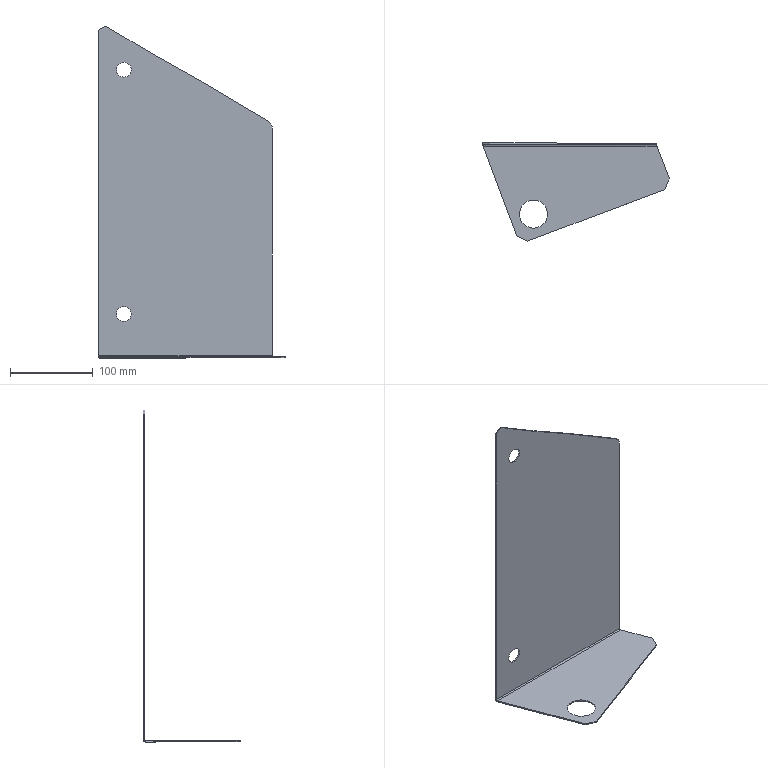Part | SolidWorks | features FlatPattern 1, SM3dBend 1, SMBaseFlange 1, SheetMetal 1 | 1 solid | 28 faces | box 225.52 x 117.762 x 400.759 mm | volume 141425 mm3 | plane 17 | cylinder 9 | spline 2 | commonest cylinder face diameters 18 x4 34 x2 3 x1 6.2 x1 20 x1
STEP:
#1=CARTESIAN_POINT('',(30.6,-1.6,-363.7));
#2=VERTEX_POINT('',#1);
#3=CARTESIAN_POINT('',(30.6,-1.6,-345.7));
#4=VERTEX_POINT('',#3);
#5=CARTESIAN_POINT('',(30.6,-1.6,-354.7));
#6=DIRECTION('',(0.,1.,0.));
#7=DIRECTION('',(0.,0.,1.));
#8=AXIS2_PLACEMENT_3D('',#5,#6,#7);
#9=CIRCLE('',#8,9.);
#10=EDGE_CURVE('',#2,#4,#9,.T.);
#11=ORIENTED_EDGE('',*,*,#10,.F.);
#12=CARTESIAN_POINT('',(30.6,0.,-363.7));
#13=VERTEX_POINT('',#12);
#14=CARTESIAN_POINT('',(30.6,-1.6,-363.7));
#15=DIRECTION('',(0.,1.,0.));
#16=VECTOR('',#15,1000.);
#17=LINE('',#14,#16);
#18=EDGE_CURVE('',#2,#13,#17,.T.);
#19=ORIENTED_EDGE('',*,*,#18,.T.);
#20=CARTESIAN_POINT('',(30.6,0.,-345.7));
#21=VERTEX_POINT('',#20);
#22=CARTESIAN_POINT('',(30.6,0.,-354.7));
#23=DIRECTION('',(0.,1.,0.));
#24=DIRECTION('',(0.,0.,1.));
#25=AXIS2_PLACEMENT_3D('',#22,#23,#24);
#26=CIRCLE('',#25,9.);
#27=EDGE_CURVE('',#13,#21,#26,.T.);
#28=ORIENTED_EDGE('',*,*,#27,.T.);
#29=CARTESIAN_POINT('',(30.6,-1.6,-345.7));
#30=DIRECTION('',(0.,1.,0.));
#31=VECTOR('',#30,1000.);
#32=LINE('',#29,#31);
#33=EDGE_CURVE('',#4,#21,#32,.T.);
#34=ORIENTED_EDGE('',*,*,#33,.F.);
#35=EDGE_LOOP('',(#11,#19,#28,#34));
#36=FACE_OUTER_BOUND('',#35,.T.);
#37=CARTESIAN_POINT('',(30.6,-1.6,-354.7));
#38=DIRECTION('',(0.,1.,0.));
#39=DIRECTION('',(0.,0.,1.));
#40=AXIS2_PLACEMENT_3D('',#37,#38,#39);
#41=CYLINDRICAL_SURFACE('',#40,9.);
#42=ADVANCED_FACE('',(#36),#41,.F.);
#43=CARTESIAN_POINT('',(30.6,-1.6,-68.7));
#44=VERTEX_POINT('',#43);
#45=CARTESIAN_POINT('',(30.6,-1.6,-50.7));
#46=VERTEX_POINT('',#45);
#47=CARTESIAN_POINT('',(30.6,-1.6,-59.7));
#48=DIRECTION('',(0.,1.,0.));
#49=DIRECTION('',(0.,0.,1.));
#50=AXIS2_PLACEMENT_3D('',#47,#48,#49);
#51=CIRCLE('',#50,9.);
#52=EDGE_CURVE('',#44,#46,#51,.T.);
#53=ORIENTED_EDGE('',*,*,#52,.F.);
#54=CARTESIAN_POINT('',(30.6,0.,-68.7));
#55=VERTEX_POINT('',#54);
#56=CARTESIAN_POINT('',(30.6,-1.6,-68.7));
#57=DIRECTION('',(0.,1.,0.));
#58=VECTOR('',#57,1000.);
#59=LINE('',#56,#58);
#60=EDGE_CURVE('',#44,#55,#59,.T.);
#61=ORIENTED_EDGE('',*,*,#60,.T.);
#62=CARTESIAN_POINT('',(30.6,0.,-50.7));
#63=VERTEX_POINT('',#62);
#64=CARTESIAN_POINT('',(30.6,0.,-59.7));
#65=DIRECTION('',(0.,1.,0.));
#66=DIRECTION('',(0.,0.,1.));
#67=AXIS2_PLACEMENT_3D('',#64,#65,#66);
#68=CIRCLE('',#67,9.);
#69=EDGE_CURVE('',#55,#63,#68,.T.);
#70=ORIENTED_EDGE('',*,*,#69,.T.);
#71=CARTESIAN_POINT('',(30.6,-1.6,-50.7));
#72=DIRECTION('',(0.,1.,0.));
#73=VECTOR('',#72,1000.);
#74=LINE('',#71,#73);
#75=EDGE_CURVE('',#46,#63,#74,.T.);
#76=ORIENTED_EDGE('',*,*,#75,.F.);
#77=EDGE_LOOP('',(#53,#61,#70,#76));
#78=FACE_OUTER_BOUND('',#77,.T.);
#79=CARTESIAN_POINT('',(30.6,-1.6,-59.7));
#80=DIRECTION('',(0.,1.,0.));
#81=DIRECTION('',(0.,0.,1.));
#82=AXIS2_PLACEMENT_3D('',#79,#80,#81);
#83=CYLINDRICAL_SURFACE('',#82,9.);
#84=ADVANCED_FACE('',(#78),#83,.F.);
#85=CARTESIAN_POINT('',(61.459,-102.219,-406.159));
#86=VERTEX_POINT('',#85);
#87=CARTESIAN_POINT('',(61.459,-68.219,-406.159));
#88=VERTEX_POINT('',#87);
#89=CARTESIAN_POINT('',(61.459,-85.219,-406.159));
#90=DIRECTION('',(0.,0.,-1.));
#91=DIRECTION('',(0.,1.,0.));
#92=AXIS2_PLACEMENT_3D('',#89,#90,#91);
#93=CIRCLE('',#92,17.);
#94=EDGE_CURVE('',#86,#88,#93,.T.);
#95=ORIENTED_EDGE('',*,*,#94,.F.);
#96=CARTESIAN_POINT('',(61.459,-102.219,-407.759));
#97=VERTEX_POINT('',#96);
#98=CARTESIAN_POINT('',(61.459,-102.219,-406.159));
#99=DIRECTION('',(0.,0.,-1.));
#100=VECTOR('',#99,1000.);
#101=LINE('',#98,#100);
#102=EDGE_CURVE('',#86,#97,#101,.T.);
#103=ORIENTED_EDGE('',*,*,#102,.T.);
#104=CARTESIAN_POINT('',(61.459,-68.219,-407.759));
#105=VERTEX_POINT('',#104);
#106=CARTESIAN_POINT('',(61.459,-85.219,-407.759));
#107=DIRECTION('',(0.,0.,-1.));
#108=DIRECTION('',(0.,1.,0.));
#109=AXIS2_PLACEMENT_3D('',#106,#107,#108);
#110=CIRCLE('',#109,17.);
#111=EDGE_CURVE('',#97,#105,#110,.T.);
#112=ORIENTED_EDGE('',*,*,#111,.T.);
#113=CARTESIAN_POINT('',(61.459,-68.219,-406.159));
#114=DIRECTION('',(0.,0.,-1.));
#115=VECTOR('',#114,1000.);
#116=LINE('',#113,#115);
#117=EDGE_CURVE('',#88,#105,#116,.T.);
#118=ORIENTED_EDGE('',*,*,#117,.F.);
#119=EDGE_LOOP('',(#95,#103,#112,#118));
#120=FACE_OUTER_BOUND('',#119,.T.);
#121=CARTESIAN_POINT('',(61.459,-85.219,-406.159));
#122=DIRECTION('',(0.,0.,-1.));
#123=DIRECTION('',(0.,1.,0.));
#124=AXIS2_PLACEMENT_3D('',#121,#122,#123);
#125=CYLINDRICAL_SURFACE('',#124,17.);
#126=ADVANCED_FACE('',(#120),#125,.F.);
#127=CARTESIAN_POINT('',(61.459,-85.219,-407.759));
#128=DIRECTION('',(0.,0.,-1.));
#129=DIRECTION('',(0.,1.,0.));
#130=AXIS2_PLACEMENT_3D('',#127,#128,#129);
#131=CIRCLE('',#130,17.);
#132=EDGE_CURVE('',#105,#97,#131,.T.);
#133=ORIENTED_EDGE('',*,*,#132,.F.);
#134=ORIENTED_EDGE('',*,*,#111,.F.);
#135=EDGE_LOOP('',(#133,#134));
#136=FACE_BOUND('',#135,.T.);
#137=CARTESIAN_POINT('',(41.582,-111.919,-407.759));
#138=VERTEX_POINT('',#137);
#139=CARTESIAN_POINT('',(0.6841,-3.1,-407.759));
#140=VERTEX_POINT('',#139);
#141=CARTESIAN_POINT('',(0.,-1.28,-407.759));
#142=DIRECTION('',(-0.3518,0.9361,0.));
#143=VECTOR('',#142,1000.);
#144=LINE('',#141,#143);
#145=EDGE_CURVE('',#138,#140,#144,.T.);
#146=ORIENTED_EDGE('',*,*,#145,.T.);
#147=CARTESIAN_POINT('',(210.604,-3.1,-407.759));
#148=VERTEX_POINT('',#147);
#149=CARTESIAN_POINT('',(199.92,-3.1,-407.759));
#150=DIRECTION('',(1.,0.,0.));
#151=VECTOR('',#150,1000.);
#152=LINE('',#149,#151);
#153=EDGE_CURVE('',#140,#148,#152,.T.);
#154=ORIENTED_EDGE('',*,*,#153,.T.);
#155=CARTESIAN_POINT('',(225.52,-42.789,-407.759));
#156=VERTEX_POINT('',#155);
#157=CARTESIAN_POINT('',(225.52,-42.789,-407.759));
#158=DIRECTION('',(0.3518,-0.9361,0.));
#159=VECTOR('',#158,1000.);
#160=LINE('',#157,#159);
#161=EDGE_CURVE('',#148,#156,#160,.T.);
#162=ORIENTED_EDGE('',*,*,#161,.T.);
#163=CARTESIAN_POINT('',(219.678,-55.668,-407.759));
#164=VERTEX_POINT('',#163);
#165=CARTESIAN_POINT('',(219.678,-55.668,-407.759));
#166=DIRECTION('',(-0.4131,-0.9107,0.));
#167=VECTOR('',#166,1000.);
#168=LINE('',#165,#167);
#169=EDGE_CURVE('',#156,#164,#168,.T.);
#170=ORIENTED_EDGE('',*,*,#169,.T.);
#171=CARTESIAN_POINT('',(54.461,-117.762,-407.759));
#172=VERTEX_POINT('',#171);
#173=CARTESIAN_POINT('',(54.461,-117.762,-407.759));
#174=DIRECTION('',(-0.9361,-0.3518,0.));
#175=VECTOR('',#174,1000.);
#176=LINE('',#173,#175);
#177=EDGE_CURVE('',#164,#172,#176,.T.);
#178=ORIENTED_EDGE('',*,*,#177,.T.);
#179=CARTESIAN_POINT('',(41.582,-111.919,-407.759));
#180=DIRECTION('',(-0.9107,0.4131,0.));
#181=VECTOR('',#180,1000.);
#182=LINE('',#179,#181);
#183=EDGE_CURVE('',#172,#138,#182,.T.);
#184=ORIENTED_EDGE('',*,*,#183,.T.);
#185=EDGE_LOOP('',(#146,#154,#162,#170,#178,#184));
#186=FACE_OUTER_BOUND('',#185,.T.);
#187=CARTESIAN_POINT('',(199.92,274.236,-407.759));
#188=DIRECTION('',(0.,0.,1.));
#189=DIRECTION('',(0.,-1.,0.));
#190=AXIS2_PLACEMENT_3D('',#187,#188,#189);
#191=PLANE('',#190);
#192=ADVANCED_FACE('',(#136,#186),#191,.F.);
#193=ORIENTED_EDGE('',*,*,#183,.F.);
#194=CARTESIAN_POINT('',(54.461,-117.762,-406.159));
#195=VERTEX_POINT('',#194);
#196=CARTESIAN_POINT('',(54.461,-117.762,-406.159));
#197=DIRECTION('',(0.,0.,-1.));
#198=VECTOR('',#197,1000.);
#199=LINE('',#196,#198);
#200=EDGE_CURVE('',#195,#172,#199,.T.);
#201=ORIENTED_EDGE('',*,*,#200,.F.);
#202=CARTESIAN_POINT('',(41.582,-111.919,-406.159));
#203=VERTEX_POINT('',#202);
#204=CARTESIAN_POINT('',(41.582,-111.919,-406.159));
#205=DIRECTION('',(-0.9107,0.4131,0.));
#206=VECTOR('',#205,1000.);
#207=LINE('',#204,#206);
#208=EDGE_CURVE('',#195,#203,#207,.T.);
#209=ORIENTED_EDGE('',*,*,#208,.T.);
#210=CARTESIAN_POINT('',(41.582,-111.919,-406.159));
#211=DIRECTION('',(0.,0.,-1.));
#212=VECTOR('',#211,1000.);
#213=LINE('',#210,#212);
#214=EDGE_CURVE('',#203,#138,#213,.T.);
#215=ORIENTED_EDGE('',*,*,#214,.T.);
#216=EDGE_LOOP('',(#193,#201,#209,#215));
#217=FACE_OUTER_BOUND('',#216,.T.);
#218=CARTESIAN_POINT('',(41.582,-111.919,-406.159));
#219=DIRECTION('',(-0.4131,-0.9107,0.));
#220=DIRECTION('',(-0.9107,0.4131,0.));
#221=AXIS2_PLACEMENT_3D('',#218,#219,#220);
#222=PLANE('',#221);
#223=ADVANCED_FACE('',(#217),#222,.T.);
#224=ORIENTED_EDGE('',*,*,#177,.F.);
#225=CARTESIAN_POINT('',(219.678,-55.668,-406.159));
#226=VERTEX_POINT('',#225);
#227=CARTESIAN_POINT('',(219.678,-55.668,-406.159));
#228=DIRECTION('',(0.,0.,-1.));
#229=VECTOR('',#228,1000.);
#230=LINE('',#227,#229);
#231=EDGE_CURVE('',#226,#164,#230,.T.);
#232=ORIENTED_EDGE('',*,*,#231,.F.);
#233=CARTESIAN_POINT('',(54.461,-117.762,-406.159));
#234=DIRECTION('',(-0.9361,-0.3518,0.));
#235=VECTOR('',#234,1000.);
#236=LINE('',#233,#235);
#237=EDGE_CURVE('',#226,#195,#236,.T.);
#238=ORIENTED_EDGE('',*,*,#237,.T.);
#239=ORIENTED_EDGE('',*,*,#200,.T.);
#240=EDGE_LOOP('',(#224,#232,#238,#239));
#241=FACE_OUTER_BOUND('',#240,.T.);
#242=CARTESIAN_POINT('',(54.461,-117.762,-406.159));
#243=DIRECTION('',(0.3518,-0.9361,0.));
#244=DIRECTION('',(-0.9361,-0.3518,0.));
#245=AXIS2_PLACEMENT_3D('',#242,#243,#244);
#246=PLANE('',#245);
#247=ADVANCED_FACE('',(#241),#246,.T.);
#248=ORIENTED_EDGE('',*,*,#169,.F.);
#249=CARTESIAN_POINT('',(225.52,-42.789,-406.159));
#250=VERTEX_POINT('',#249);
#251=CARTESIAN_POINT('',(225.52,-42.789,-406.159));
#252=DIRECTION('',(0.,0.,-1.));
#253=VECTOR('',#252,1000.);
#254=LINE('',#251,#253);
#255=EDGE_CURVE('',#250,#156,#254,.T.);
#256=ORIENTED_EDGE('',*,*,#255,.F.);
#257=CARTESIAN_POINT('',(219.678,-55.668,-406.159));
#258=DIRECTION('',(-0.4131,-0.9107,0.));
#259=VECTOR('',#258,1000.);
#260=LINE('',#257,#259);
#261=EDGE_CURVE('',#250,#226,#260,.T.);
#262=ORIENTED_EDGE('',*,*,#261,.T.);
#263=ORIENTED_EDGE('',*,*,#231,.T.);
#264=EDGE_LOOP('',(#248,#256,#262,#263));
#265=FACE_OUTER_BOUND('',#264,.T.);
#266=CARTESIAN_POINT('',(219.678,-55.668,-406.159));
#267=DIRECTION('',(0.9107,-0.4131,0.));
#268=DIRECTION('',(-0.4131,-0.9107,0.));
#269=AXIS2_PLACEMENT_3D('',#266,#267,#268);
#270=PLANE('',#269);
#271=ADVANCED_FACE('',(#265),#270,.T.);
#272=CARTESIAN_POINT('',(210.604,-3.1,-406.159));
#273=VERTEX_POINT('',#272);
#274=CARTESIAN_POINT('',(210.604,-3.1,-406.159));
#275=CARTESIAN_POINT('',(210.604,-3.1,-407.759));
#276=B_SPLINE_CURVE_WITH_KNOTS('',1,(#274,#275),.UNSPECIFIED.,.F.,.F.,(2,2),(0.,1.),.UNSPECIFIED.);
#277=EDGE_CURVE('',#273,#148,#276,.T.);
#278=ORIENTED_EDGE('',*,*,#277,.F.);
#279=CARTESIAN_POINT('',(225.52,-42.789,-406.159));
#280=DIRECTION('',(0.3518,-0.9361,0.));
#281=VECTOR('',#280,1000.);
#282=LINE('',#279,#281);
#283=EDGE_CURVE('',#273,#250,#282,.T.);
#284=ORIENTED_EDGE('',*,*,#283,.T.);
#285=ORIENTED_EDGE('',*,*,#255,.T.);
#286=ORIENTED_EDGE('',*,*,#161,.F.);
#287=EDGE_LOOP('',(#278,#284,#285,#286));
#288=FACE_OUTER_BOUND('',#287,.T.);
#289=CARTESIAN_POINT('',(225.52,-42.789,-406.159));
#290=DIRECTION('',(0.9361,0.3518,0.));
#291=DIRECTION('',(0.3518,-0.9361,0.));
#292=AXIS2_PLACEMENT_3D('',#289,#290,#291);
#293=PLANE('',#292);
#294=ADVANCED_FACE('',(#288),#293,.T.);
#295=CARTESIAN_POINT('',(0.6841,-3.1,-406.159));
#296=VERTEX_POINT('',#295);
#297=CARTESIAN_POINT('',(0.6841,-3.1,-407.759));
#298=CARTESIAN_POINT('',(0.6841,-3.1,-406.159));
#299=B_SPLINE_CURVE_WITH_KNOTS('',1,(#297,#298),.UNSPECIFIED.,.F.,.F.,(2,2),(0.,1.),.UNSPECIFIED.);
#300=EDGE_CURVE('',#140,#296,#299,.T.);
#301=ORIENTED_EDGE('',*,*,#300,.F.);
#302=ORIENTED_EDGE('',*,*,#145,.F.);
#303=ORIENTED_EDGE('',*,*,#214,.F.);
#304=CARTESIAN_POINT('',(0.,-1.28,-406.159));
#305=DIRECTION('',(-0.3518,0.9361,0.));
#306=VECTOR('',#305,1000.);
#307=LINE('',#304,#306);
#308=EDGE_CURVE('',#203,#296,#307,.T.);
#309=ORIENTED_EDGE('',*,*,#308,.T.);
#310=EDGE_LOOP('',(#301,#302,#303,#309));
#311=FACE_OUTER_BOUND('',#310,.T.);
#312=CARTESIAN_POINT('',(0.,-1.28,-406.159));
#313=DIRECTION('',(-0.9361,-0.3518,0.));
#314=DIRECTION('',(-0.3518,0.9361,0.));
#315=AXIS2_PLACEMENT_3D('',#312,#313,#314);
#316=PLANE('',#315);
#317=ADVANCED_FACE('',(#311),#316,.T.);
#318=CARTESIAN_POINT('',(199.92,-3.1,-406.159));
#319=DIRECTION('',(1.,0.,0.));
#320=VECTOR('',#319,1000.);
#321=LINE('',#318,#320);
#322=EDGE_CURVE('',#296,#273,#321,.T.);
#323=ORIENTED_EDGE('',*,*,#322,.F.);
#324=ORIENTED_EDGE('',*,*,#308,.F.);
#325=ORIENTED_EDGE('',*,*,#208,.F.);
#326=ORIENTED_EDGE('',*,*,#237,.F.);
#327=ORIENTED_EDGE('',*,*,#261,.F.);
#328=ORIENTED_EDGE('',*,*,#283,.F.);
#329=EDGE_LOOP('',(#323,#324,#325,#326,#327,#328));
#330=FACE_OUTER_BOUND('',#329,.T.);
#331=CARTESIAN_POINT('',(61.459,-85.219,-406.159));
#332=DIRECTION('',(0.,0.,-1.));
#333=DIRECTION('',(0.,1.,0.));
#334=AXIS2_PLACEMENT_3D('',#331,#332,#333);
#335=CIRCLE('',#334,17.);
#336=EDGE_CURVE('',#88,#86,#335,.T.);
#337=ORIENTED_EDGE('',*,*,#336,.T.);
#338=ORIENTED_EDGE('',*,*,#94,.T.);
#339=EDGE_LOOP('',(#337,#338));
#340=FACE_BOUND('',#339,.T.);
#341=CARTESIAN_POINT('',(199.92,274.236,-406.159));
#342=DIRECTION('',(0.,0.,1.));
#343=DIRECTION('',(0.,-1.,0.));
#344=AXIS2_PLACEMENT_3D('',#341,#342,#343);
#345=PLANE('',#344);
#346=ADVANCED_FACE('',(#330,#340),#345,.T.);
#347=ORIENTED_EDGE('',*,*,#102,.F.);
#348=ORIENTED_EDGE('',*,*,#336,.F.);
#349=ORIENTED_EDGE('',*,*,#117,.T.);
#350=ORIENTED_EDGE('',*,*,#132,.T.);
#351=EDGE_LOOP('',(#347,#348,#349,#350));
#352=FACE_OUTER_BOUND('',#351,.T.);
#353=CARTESIAN_POINT('',(61.459,-85.219,-406.159));
#354=DIRECTION('',(0.,0.,-1.));
#355=DIRECTION('',(0.,1.,0.));
#356=AXIS2_PLACEMENT_3D('',#353,#354,#355);
#357=CYLINDRICAL_SURFACE('',#356,17.);
#358=ADVANCED_FACE('',(#352),#357,.F.);
#359=CARTESIAN_POINT('',(0.,0.,-11.9));
#360=VERTEX_POINT('',#359);
#361=CARTESIAN_POINT('',(8.6,0.,-7.));
#362=VERTEX_POINT('',#361);
#363=CARTESIAN_POINT('',(8.6,0.,-7.));
#364=DIRECTION('',(0.8689,0.,0.4951));
#365=VECTOR('',#364,1000.);
#366=LINE('',#363,#365);
#367=EDGE_CURVE('',#360,#362,#366,.T.);
#368=ORIENTED_EDGE('',*,*,#367,.F.);
#369=CARTESIAN_POINT('',(0.,-1.6,-11.9));
#370=VERTEX_POINT('',#369);
#371=CARTESIAN_POINT('',(0.,-1.6,-11.9));
#372=DIRECTION('',(0.,1.,0.));
#373=VECTOR('',#372,1000.);
#374=LINE('',#371,#373);
#375=EDGE_CURVE('',#370,#360,#374,.T.);
#376=ORIENTED_EDGE('',*,*,#375,.F.);
#377=CARTESIAN_POINT('',(8.6,-1.6,-7.));
#378=VERTEX_POINT('',#377);
#379=CARTESIAN_POINT('',(8.6,-1.6,-7.));
#380=DIRECTION('',(0.8689,0.,0.4951));
#381=VECTOR('',#380,1000.);
#382=LINE('',#379,#381);
#383=EDGE_CURVE('',#370,#378,#382,.T.);
#384=ORIENTED_EDGE('',*,*,#383,.T.);
#385=CARTESIAN_POINT('',(8.6,-1.6,-7.));
#386=DIRECTION('',(0.,1.,0.));
#387=VECTOR('',#386,1000.);
#388=LINE('',#385,#387);
#389=EDGE_CURVE('',#378,#362,#388,.T.);
#390=ORIENTED_EDGE('',*,*,#389,.T.);
#391=EDGE_LOOP('',(#368,#376,#384,#390));
#392=FACE_OUTER_BOUND('',#391,.T.);
#393=CARTESIAN_POINT('',(8.6,-1.6,-7.));
#394=DIRECTION('',(-0.4951,0.,0.8689));
#395=DIRECTION('',(0.8689,0.,0.4951));
#396=AXIS2_PLACEMENT_3D('',#393,#394,#395);
#397=PLANE('',#396);
#398=ADVANCED_FACE('',(#392),#397,.T.);
#399=CARTESIAN_POINT('',(66.,0.,-41.2));
#400=VERTEX_POINT('',#399);
#401=CARTESIAN_POINT('',(66.,0.,-41.2));
#402=DIRECTION('',(0.8591,0.,-0.5119));
#403=VECTOR('',#402,1000.);
#404=LINE('',#401,#403);
#405=EDGE_CURVE('',#362,#400,#404,.T.);
#406=ORIENTED_EDGE('',*,*,#405,.F.);
#407=ORIENTED_EDGE('',*,*,#389,.F.);
#408=CARTESIAN_POINT('',(66.,-1.6,-41.2));
#409=VERTEX_POINT('',#408);
#410=CARTESIAN_POINT('',(66.,-1.6,-41.2));
#411=DIRECTION('',(0.8591,0.,-0.5119));
#412=VECTOR('',#411,1000.);
#413=LINE('',#410,#412);
#414=EDGE_CURVE('',#378,#409,#413,.T.);
#415=ORIENTED_EDGE('',*,*,#414,.T.);
#416=CARTESIAN_POINT('',(66.,-1.6,-41.2));
#417=DIRECTION('',(0.,1.,0.));
#418=VECTOR('',#417,1000.);
#419=LINE('',#416,#418);
#420=EDGE_CURVE('',#409,#400,#419,.T.);
#421=ORIENTED_EDGE('',*,*,#420,.T.);
#422=EDGE_LOOP('',(#406,#407,#415,#421));
#423=FACE_OUTER_BOUND('',#422,.T.);
#424=CARTESIAN_POINT('',(66.,-1.6,-41.2));
#425=DIRECTION('',(0.5119,0.,0.8591));
#426=DIRECTION('',(0.8591,0.,-0.5119));
#427=AXIS2_PLACEMENT_3D('',#424,#425,#426);
#428=PLANE('',#427);
#429=ADVANCED_FACE('',(#423),#428,.T.);
#430=CARTESIAN_POINT('',(125.28,0.,-74.6));
#431=VERTEX_POINT('',#430);
#432=CARTESIAN_POINT('',(125.28,0.,-74.6));
#433=DIRECTION('',(0.8712,0.,-0.4909));
#434=VECTOR('',#433,1000.);
#435=LINE('',#432,#434);
#436=EDGE_CURVE('',#400,#431,#435,.T.);
#437=ORIENTED_EDGE('',*,*,#436,.F.);
#438=ORIENTED_EDGE('',*,*,#420,.F.);
#439=CARTESIAN_POINT('',(125.28,-1.6,-74.6));
#440=VERTEX_POINT('',#439);
#441=CARTESIAN_POINT('',(125.28,-1.6,-74.6));
#442=DIRECTION('',(0.8712,0.,-0.4909));
#443=VECTOR('',#442,1000.);
#444=LINE('',#441,#443);
#445=EDGE_CURVE('',#409,#440,#444,.T.);
#446=ORIENTED_EDGE('',*,*,#445,.T.);
#447=CARTESIAN_POINT('',(125.28,-1.6,-74.6));
#448=DIRECTION('',(0.,1.,0.));
#449=VECTOR('',#448,1000.);
#450=LINE('',#447,#449);
#451=EDGE_CURVE('',#440,#431,#450,.T.);
#452=ORIENTED_EDGE('',*,*,#451,.T.);
#453=EDGE_LOOP('',(#437,#438,#446,#452));
#454=FACE_OUTER_BOUND('',#453,.T.);
#455=CARTESIAN_POINT('',(125.28,-1.6,-74.6));
#456=DIRECTION('',(0.4909,0.,0.8712));
#457=DIRECTION('',(0.8712,0.,-0.4909));
#458=AXIS2_PLACEMENT_3D('',#455,#456,#457);
#459=PLANE('',#458);
#460=ADVANCED_FACE('',(#454),#459,.T.);
#461=CARTESIAN_POINT('',(205.036,0.,-122.092));
#462=VERTEX_POINT('',#461);
#463=CARTESIAN_POINT('',(205.036,0.,-122.092));
#464=DIRECTION('',(0.8592,0.,-0.5116));
#465=VECTOR('',#464,1000.);
#466=LINE('',#463,#465);
#467=EDGE_CURVE('',#431,#462,#466,.T.);
#468=ORIENTED_EDGE('',*,*,#467,.F.);
#469=ORIENTED_EDGE('',*,*,#451,.F.);
#470=CARTESIAN_POINT('',(205.036,-1.6,-122.092));
#471=VERTEX_POINT('',#470);
#472=CARTESIAN_POINT('',(205.036,-1.6,-122.092));
#473=DIRECTION('',(0.8592,0.,-0.5116));
#474=VECTOR('',#473,1000.);
#475=LINE('',#472,#474);
#476=EDGE_CURVE('',#440,#471,#475,.T.);
#477=ORIENTED_EDGE('',*,*,#476,.T.);
#478=CARTESIAN_POINT('',(205.036,-1.6,-122.092));
#479=DIRECTION('',(0.,1.,0.));
#480=VECTOR('',#479,1000.);
#481=LINE('',#478,#480);
#482=EDGE_CURVE('',#471,#462,#481,.T.);
#483=ORIENTED_EDGE('',*,*,#482,.T.);
#484=EDGE_LOOP('',(#468,#469,#477,#483));
#485=FACE_OUTER_BOUND('',#484,.T.);
#486=CARTESIAN_POINT('',(205.036,-1.6,-122.092));
#487=DIRECTION('',(0.5116,0.,0.8592));
#488=DIRECTION('',(0.8592,0.,-0.5116));
#489=AXIS2_PLACEMENT_3D('',#486,#487,#488);
#490=PLANE('',#489);
#491=ADVANCED_FACE('',(#485),#490,.T.);
#492=CARTESIAN_POINT('',(209.92,0.,-130.684));
#493=VERTEX_POINT('',#492);
#494=CARTESIAN_POINT('',(199.92,0.,-130.684));
#495=DIRECTION('',(0.,1.,0.));
#496=DIRECTION('',(0.,0.,-1.));
#497=AXIS2_PLACEMENT_3D('',#494,#495,#496);
#498=CIRCLE('',#497,10.);
#499=EDGE_CURVE('',#462,#493,#498,.T.);
#500=ORIENTED_EDGE('',*,*,#499,.F.);
#501=ORIENTED_EDGE('',*,*,#482,.F.);
#502=CARTESIAN_POINT('',(209.92,-1.6,-130.684));
#503=VERTEX_POINT('',#502);
#504=CARTESIAN_POINT('',(199.92,-1.6,-130.684));
#505=DIRECTION('',(0.,1.,0.));
#506=DIRECTION('',(0.,0.,-1.));
#507=AXIS2_PLACEMENT_3D('',#504,#505,#506);
#508=CIRCLE('',#507,10.);
#509=EDGE_CURVE('',#471,#503,#508,.T.);
#510=ORIENTED_EDGE('',*,*,#509,.T.);
#511=CARTESIAN_POINT('',(209.92,-1.6,-130.684));
#512=DIRECTION('',(0.,1.,0.));
#513=VECTOR('',#512,1000.);
#514=LINE('',#511,#513);
#515=EDGE_CURVE('',#503,#493,#514,.T.);
#516=ORIENTED_EDGE('',*,*,#515,.T.);
#517=EDGE_LOOP('',(#500,#501,#510,#516));
#518=FACE_OUTER_BOUND('',#517,.T.);
#519=CARTESIAN_POINT('',(199.92,-1.6,-130.684));
#520=DIRECTION('',(0.,1.,0.));
#521=DIRECTION('',(0.,0.,1.));
#522=AXIS2_PLACEMENT_3D('',#519,#520,#521);
#523=CYLINDRICAL_SURFACE('',#522,10.);
#524=ADVANCED_FACE('',(#518),#523,.T.);
#525=ORIENTED_EDGE('',*,*,#60,.F.);
#526=CARTESIAN_POINT('',(30.6,-1.6,-59.7));
#527=DIRECTION('',(0.,1.,0.));
#528=DIRECTION('',(0.,0.,1.));
#529=AXIS2_PLACEMENT_3D('',#526,#527,#528);
#530=CIRCLE('',#529,9.);
#531=EDGE_CURVE('',#46,#44,#530,.T.);
#532=ORIENTED_EDGE('',*,*,#531,.F.);
#533=ORIENTED_EDGE('',*,*,#75,.T.);
#534=CARTESIAN_POINT('',(30.6,0.,-59.7));
#535=DIRECTION('',(0.,1.,0.));
#536=DIRECTION('',(0.,0.,1.));
#537=AXIS2_PLACEMENT_3D('',#534,#535,#536);
#538=CIRCLE('',#537,9.);
#539=EDGE_CURVE('',#63,#55,#538,.T.);
#540=ORIENTED_EDGE('',*,*,#539,.T.);
#541=EDGE_LOOP('',(#525,#532,#533,#540));
#542=FACE_OUTER_BOUND('',#541,.T.);
#543=CARTESIAN_POINT('',(30.6,-1.6,-59.7));
#544=DIRECTION('',(0.,1.,0.));
#545=DIRECTION('',(0.,0.,1.));
#546=AXIS2_PLACEMENT_3D('',#543,#544,#545);
#547=CYLINDRICAL_SURFACE('',#546,9.);
#548=ADVANCED_FACE('',(#542),#547,.F.);
#549=ORIENTED_EDGE('',*,*,#18,.F.);
#550=CARTESIAN_POINT('',(30.6,-1.6,-354.7));
#551=DIRECTION('',(0.,1.,0.));
#552=DIRECTION('',(0.,0.,1.));
#553=AXIS2_PLACEMENT_3D('',#550,#551,#552);
#554=CIRCLE('',#553,9.);
#555=EDGE_CURVE('',#4,#2,#554,.T.);
#556=ORIENTED_EDGE('',*,*,#555,.F.);
#557=ORIENTED_EDGE('',*,*,#33,.T.);
#558=CARTESIAN_POINT('',(30.6,0.,-354.7));
#559=DIRECTION('',(0.,1.,0.));
#560=DIRECTION('',(0.,0.,1.));
#561=AXIS2_PLACEMENT_3D('',#558,#559,#560);
#562=CIRCLE('',#561,9.);
#563=EDGE_CURVE('',#21,#13,#562,.T.);
#564=ORIENTED_EDGE('',*,*,#563,.T.);
#565=EDGE_LOOP('',(#549,#556,#557,#564));
#566=FACE_OUTER_BOUND('',#565,.T.);
#567=CARTESIAN_POINT('',(30.6,-1.6,-354.7));
#568=DIRECTION('',(0.,1.,0.));
#569=DIRECTION('',(0.,0.,1.));
#570=AXIS2_PLACEMENT_3D('',#567,#568,#569);
#571=CYLINDRICAL_SURFACE('',#570,9.);
#572=ADVANCED_FACE('',(#566),#571,.F.);
#573=ORIENTED_EDGE('',*,*,#555,.T.);
#574=ORIENTED_EDGE('',*,*,#10,.T.);
#575=EDGE_LOOP('',(#573,#574));
#576=FACE_BOUND('',#575,.T.);
#577=ORIENTED_EDGE('',*,*,#531,.T.);
#578=ORIENTED_EDGE('',*,*,#52,.T.);
#579=EDGE_LOOP('',(#577,#578));
#580=FACE_BOUND('',#579,.T.);
#581=CARTESIAN_POINT('',(0.,-1.6,-404.659));
#582=VERTEX_POINT('',#581);
#583=CARTESIAN_POINT('',(0.,-1.6,-11.9));
#584=DIRECTION('',(0.,0.,1.));
#585=VECTOR('',#584,1000.);
#586=LINE('',#583,#585);
#587=EDGE_CURVE('',#582,#370,#586,.T.);
#588=ORIENTED_EDGE('',*,*,#587,.F.);
#589=CARTESIAN_POINT('',(209.92,-1.6,-404.659));
#590=VERTEX_POINT('',#589);
#591=CARTESIAN_POINT('',(199.92,-1.6,-404.659));
#592=DIRECTION('',(1.,0.,0.));
#593=VECTOR('',#592,1000.);
#594=LINE('',#591,#593);
#595=EDGE_CURVE('',#582,#590,#594,.T.);
#596=ORIENTED_EDGE('',*,*,#595,.T.);
#597=CARTESIAN_POINT('',(209.92,-1.6,-406.2));
#598=DIRECTION('',(0.,0.,-1.));
#599=VECTOR('',#598,1000.);
#600=LINE('',#597,#599);
#601=EDGE_CURVE('',#503,#590,#600,.T.);
#602=ORIENTED_EDGE('',*,*,#601,.F.);
#603=ORIENTED_EDGE('',*,*,#509,.F.);
#604=ORIENTED_EDGE('',*,*,#476,.F.);
#605=ORIENTED_EDGE('',*,*,#445,.F.);
#606=ORIENTED_EDGE('',*,*,#414,.F.);
#607=ORIENTED_EDGE('',*,*,#383,.F.);
#608=EDGE_LOOP('',(#588,#596,#602,#603,#604,#605,#606,#607));
#609=FACE_OUTER_BOUND('',#608,.T.);
#610=CARTESIAN_POINT('',(199.92,-1.6,-130.684));
#611=DIRECTION('',(0.,-1.,0.));
#612=DIRECTION('',(0.,0.,-1.));
#613=AXIS2_PLACEMENT_3D('',#610,#611,#612);
#614=PLANE('',#613);
#615=ADVANCED_FACE('',(#576,#580,#609),#614,.T.);
#616=ORIENTED_EDGE('',*,*,#601,.T.);
#617=CARTESIAN_POINT('',(209.92,0.,-404.659));
#618=VERTEX_POINT('',#617);
#619=CARTESIAN_POINT('',(209.92,-1.6,-404.659));
#620=DIRECTION('',(0.,1.,0.));
#621=VECTOR('',#620,1000.);
#622=LINE('',#619,#621);
#623=EDGE_CURVE('',#590,#618,#622,.T.);
#624=ORIENTED_EDGE('',*,*,#623,.T.);
#625=CARTESIAN_POINT('',(209.92,0.,-406.2));
#626=DIRECTION('',(0.,0.,-1.));
#627=VECTOR('',#626,1000.);
#628=LINE('',#625,#627);
#629=EDGE_CURVE('',#493,#618,#628,.T.);
#630=ORIENTED_EDGE('',*,*,#629,.F.);
#631=ORIENTED_EDGE('',*,*,#515,.F.);
#632=EDGE_LOOP('',(#616,#624,#630,#631));
#633=FACE_OUTER_BOUND('',#632,.T.);
#634=CARTESIAN_POINT('',(209.92,-1.6,-406.2));
#635=DIRECTION('',(1.,0.,0.));
#636=DIRECTION('',(0.,0.,-1.));
#637=AXIS2_PLACEMENT_3D('',#634,#635,#636);
#638=PLANE('',#637);
#639=ADVANCED_FACE('',(#633),#638,.T.);
#640=CARTESIAN_POINT('',(0.,0.,-404.659));
#641=VERTEX_POINT('',#640);
#642=CARTESIAN_POINT('',(199.92,0.,-404.659));
#643=DIRECTION('',(1.,0.,0.));
#644=VECTOR('',#643,1000.);
#645=LINE('',#642,#644);
#646=EDGE_CURVE('',#641,#618,#645,.T.);
#647=ORIENTED_EDGE('',*,*,#646,.F.);
#648=CARTESIAN_POINT('',(0.,0.,-11.9));
#649=DIRECTION('',(0.,0.,1.));
#650=VECTOR('',#649,1000.);
#651=LINE('',#648,#650);
#652=EDGE_CURVE('',#641,#360,#651,.T.);
#653=ORIENTED_EDGE('',*,*,#652,.T.);
#654=ORIENTED_EDGE('',*,*,#367,.T.);
#655=ORIENTED_EDGE('',*,*,#405,.T.);
#656=ORIENTED_EDGE('',*,*,#436,.T.);
#657=ORIENTED_EDGE('',*,*,#467,.T.);
#658=ORIENTED_EDGE('',*,*,#499,.T.);
#659=ORIENTED_EDGE('',*,*,#629,.T.);
#660=EDGE_LOOP('',(#647,#653,#654,#655,#656,#657,#658,#659));
#661=FACE_OUTER_BOUND('',#660,.T.);
#662=ORIENTED_EDGE('',*,*,#539,.F.);
#663=ORIENTED_EDGE('',*,*,#69,.F.);
#664=EDGE_LOOP('',(#662,#663));
#665=FACE_BOUND('',#664,.T.);
#666=ORIENTED_EDGE('',*,*,#563,.F.);
#667=ORIENTED_EDGE('',*,*,#27,.F.);
#668=EDGE_LOOP('',(#666,#667));
#669=FACE_BOUND('',#668,.T.);
#670=CARTESIAN_POINT('',(199.92,0.,-130.684));
#671=DIRECTION('',(0.,-1.,0.));
#672=DIRECTION('',(0.,0.,-1.));
#673=AXIS2_PLACEMENT_3D('',#670,#671,#672);
#674=PLANE('',#673);
#675=ADVANCED_FACE('',(#661,#665,#669),#674,.F.);
#676=ORIENTED_EDGE('',*,*,#652,.F.);
#677=CARTESIAN_POINT('',(0.,-1.6,-404.659));
#678=DIRECTION('',(0.,-1.,0.));
#679=VECTOR('',#678,1000.);
#680=LINE('',#677,#679);
#681=EDGE_CURVE('',#641,#582,#680,.T.);
#682=ORIENTED_EDGE('',*,*,#681,.T.);
#683=ORIENTED_EDGE('',*,*,#587,.T.);
#684=ORIENTED_EDGE('',*,*,#375,.T.);
#685=EDGE_LOOP('',(#676,#682,#683,#684));
#686=FACE_OUTER_BOUND('',#685,.T.);
#687=CARTESIAN_POINT('',(0.,-1.6,-11.9));
#688=DIRECTION('',(-1.,0.,0.));
#689=DIRECTION('',(0.,0.,1.));
#690=AXIS2_PLACEMENT_3D('',#687,#688,#689);
#691=PLANE('',#690);
#692=ADVANCED_FACE('',(#686),#691,.T.);
#693=ORIENTED_EDGE('',*,*,#681,.F.);
#694=CARTESIAN_POINT('',(0.,-0.77,-406.703));
#695=VERTEX_POINT('',#694);
#696=CARTESIAN_POINT('',(0.,-3.1,-404.659));
#697=DIRECTION('',(-1.,0.,0.));
#698=DIRECTION('',(0.,0.,-1.));
#699=AXIS2_PLACEMENT_3D('',#696,#697,#698);
#700=CIRCLE('',#699,3.1);
#701=EDGE_CURVE('',#641,#695,#700,.T.);
#702=ORIENTED_EDGE('',*,*,#701,.T.);
#703=CARTESIAN_POINT('',(0.,-1.973,-405.648));
#704=VERTEX_POINT('',#703);
#705=CARTESIAN_POINT('',(0.,-0.77,-406.703));
#706=CARTESIAN_POINT('',(0.,-1.171,-406.352));
#707=CARTESIAN_POINT('',(0.,-1.572,-406.));
#708=CARTESIAN_POINT('',(0.,-1.973,-405.648));
#709=B_SPLINE_CURVE_WITH_KNOTS('',3,(#705,#706,#707,#708),.UNSPECIFIED.,.F.,.F.,(4,4),(0.,1.),.UNSPECIFIED.);
#710=EDGE_CURVE('',#695,#704,#709,.T.);
#711=ORIENTED_EDGE('',*,*,#710,.T.);
#712=CARTESIAN_POINT('',(0.,-3.1,-404.659));
#713=DIRECTION('',(-1.,0.,0.));
#714=DIRECTION('',(0.,0.,-1.));
#715=AXIS2_PLACEMENT_3D('',#712,#713,#714);
#716=CIRCLE('',#715,1.5);
#717=EDGE_CURVE('',#582,#704,#716,.T.);
#718=ORIENTED_EDGE('',*,*,#717,.F.);
#719=EDGE_LOOP('',(#693,#702,#711,#718));
#720=FACE_OUTER_BOUND('',#719,.T.);
#721=CARTESIAN_POINT('',(0.,-3.1,-404.659));
#722=DIRECTION('',(1.,0.,0.));
#723=DIRECTION('',(0.,0.,-1.));
#724=AXIS2_PLACEMENT_3D('',#721,#722,#723);
#725=PLANE('',#724);
#726=ADVANCED_FACE('',(#720),#725,.F.);
#727=ORIENTED_EDGE('',*,*,#710,.F.);
#728=CARTESIAN_POINT('',(0.,-0.77,-406.703));
#729=CARTESIAN_POINT('',(0.114,-1.06,-407.034));
#730=CARTESIAN_POINT('',(0.228,-1.421,-407.301));
#731=CARTESIAN_POINT('',(0.456,-2.221,-407.664));
#732=CARTESIAN_POINT('',(0.57,-2.66,-407.759));
#733=CARTESIAN_POINT('',(0.6841,-3.1,-407.759));
#734=B_SPLINE_CURVE_WITH_KNOTS('',3,(#728,#729,#730,#731,#732,#733),.UNSPECIFIED.,.F.,.F.,(4,2,4),(0.,0.5,1.),.UNSPECIFIED.);
#735=EDGE_CURVE('',#695,#140,#734,.T.);
#736=ORIENTED_EDGE('',*,*,#735,.T.);
#737=ORIENTED_EDGE('',*,*,#300,.T.);
#738=CARTESIAN_POINT('',(0.,-1.973,-405.648));
#739=CARTESIAN_POINT('',(0.114,-2.113,-405.808));
#740=CARTESIAN_POINT('',(0.228,-2.287,-405.937));
#741=CARTESIAN_POINT('',(0.456,-2.675,-406.113));
#742=CARTESIAN_POINT('',(0.5701,-2.887,-406.159));
#743=CARTESIAN_POINT('',(0.6841,-3.1,-406.159));
#744=B_SPLINE_CURVE_WITH_KNOTS('',3,(#738,#739,#740,#741,#742,#743),.UNSPECIFIED.,.F.,.F.,(4,2,4),(0.,0.5,1.),.UNSPECIFIED.);
#745=EDGE_CURVE('',#704,#296,#744,.T.);
#746=ORIENTED_EDGE('',*,*,#745,.F.);
#747=EDGE_LOOP('',(#727,#736,#737,#746));
#748=FACE_OUTER_BOUND('',#747,.T.);
#749=CARTESIAN_POINT('',(0.,-0.77,-406.703));
#750=CARTESIAN_POINT('',(0.114,-1.06,-407.034));
#751=CARTESIAN_POINT('',(0.228,-1.421,-407.301));
#752=CARTESIAN_POINT('',(0.456,-2.221,-407.664));
#753=CARTESIAN_POINT('',(0.57,-2.66,-407.759));
#754=CARTESIAN_POINT('',(0.6841,-3.1,-407.759));
#755=CARTESIAN_POINT('',(0.,-1.973,-405.648));
#756=CARTESIAN_POINT('',(0.114,-2.113,-405.808));
#757=CARTESIAN_POINT('',(0.228,-2.287,-405.937));
#758=CARTESIAN_POINT('',(0.456,-2.675,-406.113));
#759=CARTESIAN_POINT('',(0.57,-2.887,-406.159));
#760=CARTESIAN_POINT('',(0.6841,-3.1,-406.159));
#761=B_SPLINE_SURFACE_WITH_KNOTS('',1,3,((#749,#750,#751,#752,#753,#754),(#755,#756,#757,#758,#759,#760)),.UNSPECIFIED.,.F.,.F.,.F.,(2,2),(4,2,4),(0.,1.),(0.,0.5,1.),.UNSPECIFIED.);
#762=ADVANCED_FACE('',(#748),#761,.F.);
#763=ORIENTED_EDGE('',*,*,#277,.T.);
#764=CARTESIAN_POINT('',(209.92,-0.77,-406.703));
#765=VERTEX_POINT('',#764);
#766=CARTESIAN_POINT('',(210.604,-3.1,-407.759));
#767=CARTESIAN_POINT('',(210.49,-2.66,-407.759));
#768=CARTESIAN_POINT('',(210.376,-2.221,-407.664));
#769=CARTESIAN_POINT('',(210.148,-1.421,-407.301));
#770=CARTESIAN_POINT('',(210.034,-1.06,-407.034));
#771=CARTESIAN_POINT('',(209.92,-0.77,-406.703));
#772=B_SPLINE_CURVE_WITH_KNOTS('',3,(#766,#767,#768,#769,#770,#771),.UNSPECIFIED.,.F.,.F.,(4,2,4),(0.,0.5,1.),.UNSPECIFIED.);
#773=EDGE_CURVE('',#148,#765,#772,.T.);
#774=ORIENTED_EDGE('',*,*,#773,.T.);
#775=CARTESIAN_POINT('',(209.92,-1.973,-405.648));
#776=VERTEX_POINT('',#775);
#777=CARTESIAN_POINT('',(209.92,-0.77,-406.703));
#778=CARTESIAN_POINT('',(209.92,-1.973,-405.648));
#779=B_SPLINE_CURVE_WITH_KNOTS('',1,(#777,#778),.UNSPECIFIED.,.F.,.F.,(2,2),(0.,1.),.UNSPECIFIED.);
#780=EDGE_CURVE('',#765,#776,#779,.T.);
#781=ORIENTED_EDGE('',*,*,#780,.T.);
#782=CARTESIAN_POINT('',(210.604,-3.1,-406.159));
#783=CARTESIAN_POINT('',(210.49,-2.887,-406.159));
#784=CARTESIAN_POINT('',(210.376,-2.675,-406.113));
#785=CARTESIAN_POINT('',(210.148,-2.287,-405.937));
#786=CARTESIAN_POINT('',(210.034,-2.113,-405.808));
#787=CARTESIAN_POINT('',(209.92,-1.973,-405.648));
#788=B_SPLINE_CURVE_WITH_KNOTS('',3,(#782,#783,#784,#785,#786,#787),.UNSPECIFIED.,.F.,.F.,(4,2,4),(0.,0.5,1.),.UNSPECIFIED.);
#789=EDGE_CURVE('',#273,#776,#788,.T.);
#790=ORIENTED_EDGE('',*,*,#789,.F.);
#791=EDGE_LOOP('',(#763,#774,#781,#790));
#792=FACE_OUTER_BOUND('',#791,.T.);
#793=CARTESIAN_POINT('',(210.604,-3.1,-407.759));
#794=CARTESIAN_POINT('',(210.49,-2.66,-407.759));
#795=CARTESIAN_POINT('',(210.376,-2.221,-407.664));
#796=CARTESIAN_POINT('',(210.148,-1.421,-407.301));
#797=CARTESIAN_POINT('',(210.034,-1.06,-407.034));
#798=CARTESIAN_POINT('',(209.92,-0.77,-406.703));
#799=CARTESIAN_POINT('',(210.604,-3.1,-406.159));
#800=CARTESIAN_POINT('',(210.49,-2.887,-406.159));
#801=CARTESIAN_POINT('',(210.376,-2.675,-406.113));
#802=CARTESIAN_POINT('',(210.148,-2.287,-405.937));
#803=CARTESIAN_POINT('',(210.034,-2.113,-405.808));
#804=CARTESIAN_POINT('',(209.92,-1.973,-405.648));
#805=B_SPLINE_SURFACE_WITH_KNOTS('',1,3,((#793,#794,#795,#796,#797,#798),(#799,#800,#801,#802,#803,#804)),.UNSPECIFIED.,.F.,.F.,.F.,(2,2),(4,2,4),(0.,1.),(0.,0.5,1.),.UNSPECIFIED.);
#806=ADVANCED_FACE('',(#792),#805,.F.);
#807=CARTESIAN_POINT('',(209.92,-3.1,-404.659));
#808=DIRECTION('',(1.,0.,0.));
#809=DIRECTION('',(0.,0.,-1.));
#810=AXIS2_PLACEMENT_3D('',#807,#808,#809);
#811=CIRCLE('',#810,3.1);
#812=EDGE_CURVE('',#765,#618,#811,.T.);
#813=ORIENTED_EDGE('',*,*,#812,.T.);
#814=ORIENTED_EDGE('',*,*,#623,.F.);
#815=CARTESIAN_POINT('',(209.92,-3.1,-404.659));
#816=DIRECTION('',(1.,0.,0.));
#817=DIRECTION('',(0.,0.,1.));
#818=AXIS2_PLACEMENT_3D('',#815,#816,#817);
#819=CIRCLE('',#818,1.5);
#820=EDGE_CURVE('',#776,#590,#819,.T.);
#821=ORIENTED_EDGE('',*,*,#820,.F.);
#822=ORIENTED_EDGE('',*,*,#780,.F.);
#823=EDGE_LOOP('',(#813,#814,#821,#822));
#824=FACE_OUTER_BOUND('',#823,.T.);
#825=CARTESIAN_POINT('',(209.92,-3.1,-404.659));
#826=DIRECTION('',(-1.,0.,0.));
#827=DIRECTION('',(0.,0.,1.));
#828=AXIS2_PLACEMENT_3D('',#825,#826,#827);
#829=PLANE('',#828);
#830=ADVANCED_FACE('',(#824),#829,.F.);
#831=ORIENTED_EDGE('',*,*,#789,.T.);
#832=ORIENTED_EDGE('',*,*,#820,.T.);
#833=ORIENTED_EDGE('',*,*,#595,.F.);
#834=ORIENTED_EDGE('',*,*,#717,.T.);
#835=ORIENTED_EDGE('',*,*,#745,.T.);
#836=ORIENTED_EDGE('',*,*,#322,.T.);
#837=EDGE_LOOP('',(#831,#832,#833,#834,#835,#836));
#838=FACE_OUTER_BOUND('',#837,.T.);
#839=CARTESIAN_POINT('',(-105.677,-3.1,-404.659));
#840=DIRECTION('',(1.,0.,0.));
#841=DIRECTION('',(0.,0.,-1.));
#842=AXIS2_PLACEMENT_3D('',#839,#840,#841);
#843=CYLINDRICAL_SURFACE('',#842,1.5);
#844=ADVANCED_FACE('',(#838),#843,.F.);
#845=ORIENTED_EDGE('',*,*,#773,.F.);
#846=ORIENTED_EDGE('',*,*,#153,.F.);
#847=ORIENTED_EDGE('',*,*,#735,.F.);
#848=ORIENTED_EDGE('',*,*,#701,.F.);
#849=ORIENTED_EDGE('',*,*,#646,.T.);
#850=ORIENTED_EDGE('',*,*,#812,.F.);
#851=EDGE_LOOP('',(#845,#846,#847,#848,#849,#850));
#852=FACE_OUTER_BOUND('',#851,.T.);
#853=CARTESIAN_POINT('',(-105.677,-3.1,-404.659));
#854=DIRECTION('',(1.,0.,0.));
#855=DIRECTION('',(0.,0.,-1.));
#856=AXIS2_PLACEMENT_3D('',#853,#854,#855);
#857=CYLINDRICAL_SURFACE('',#856,3.1);
#858=ADVANCED_FACE('',(#852),#857,.T.);
#859=CLOSED_SHELL('',(#42,#84,#126,#192,#223,#247,#271,#294,#317,#346,#358,#398,#429,#460,#491,#524,#548,#572,#615,#639,#675,#692,#726,#762,#806,#830,#844,#858));
#860=MANIFOLD_SOLID_BREP('',#859);
#861=CARTESIAN_POINT('',(0.,0.,0.));
#862=DIRECTION('',(0.,0.,1.));
#863=DIRECTION('',(1.,0.,0.));
#864=AXIS2_PLACEMENT_3D('',#861,#862,#863);
#865=(LENGTH_UNIT()NAMED_UNIT(*)SI_UNIT(.MILLI.,.METRE.));
#866=UNCERTAINTY_MEASURE_WITH_UNIT(LENGTH_MEASURE(0.00001),#865,'','');
#867=(NAMED_UNIT(*)PLANE_ANGLE_UNIT()SI_UNIT($,.RADIAN.));
#868=(NAMED_UNIT(*)SI_UNIT($,.STERADIAN.)SOLID_ANGLE_UNIT());
#869=(GEOMETRIC_REPRESENTATION_CONTEXT(3)GLOBAL_UNCERTAINTY_ASSIGNED_CONTEXT((#866))GLOBAL_UNIT_ASSIGNED_CONTEXT((#865,#867,#868))REPRESENTATION_CONTEXT('',''));
#870=ADVANCED_BREP_SHAPE_REPRESENTATION('',(#860,#864),#869);